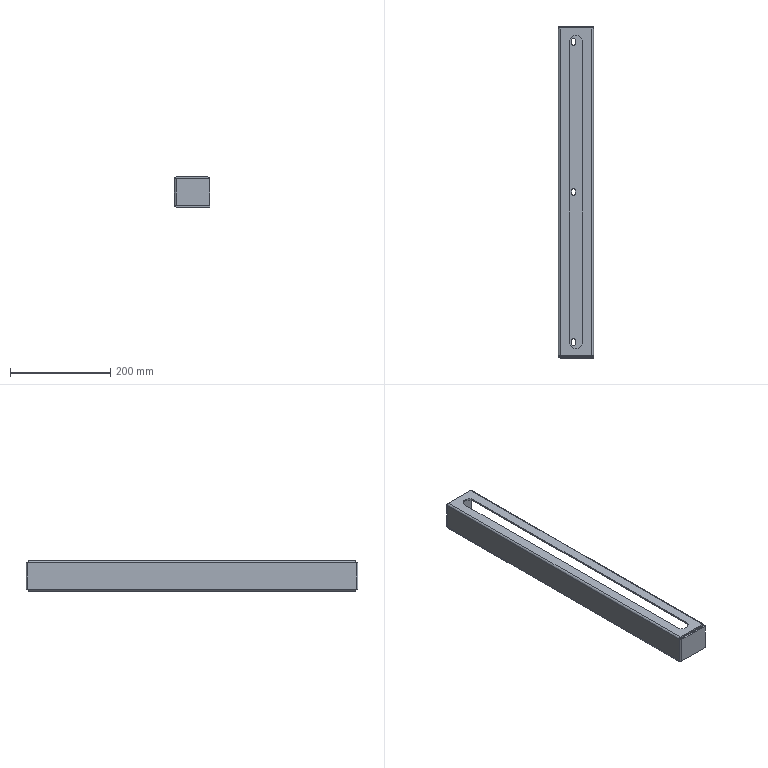Part | SolidWorks | features BaseBody 1 | 1 solid | 78 faces | box 70 x 663 x 60 mm | volume 379659 mm3 | plane 34 | cylinder 30 | cone 14 | commonest cylinder face diameters 1.473 x7 6.6 x6 14 x6 7.473 x5 3.3 x4 25 x2